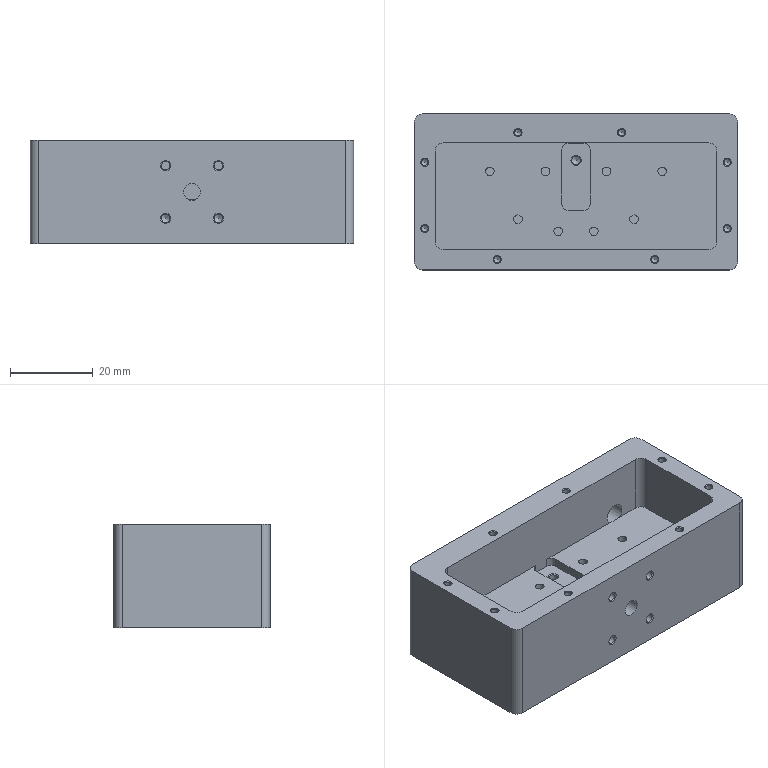Part | STEP file | 2-in-1 cavity | 1 solid | 112 faces | box 78 x 37.65 x 25 mm | volume 47258 mm3 | cylinder 44 | cone 42 | plane 26 | commonest cylinder face diameters 2.05 x13 1.6 x8 2.1 x8 4 x8 3 x4 5 x2